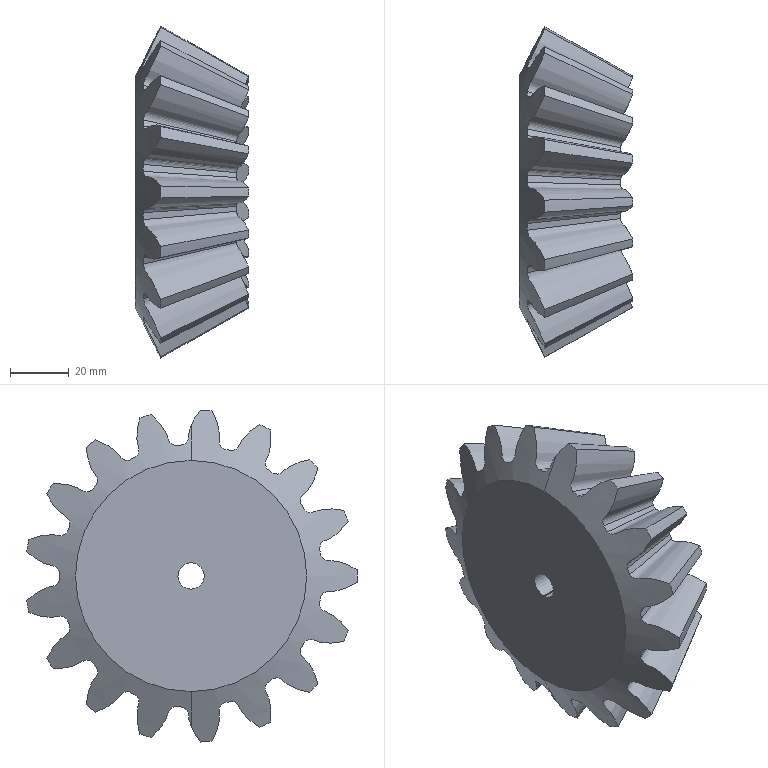Part | STEP file | Bevel gear 17×2 | 1 solid | 94 faces | box 38.391 x 112.113 x 112.556 mm | volume 206962 mm3 | spline 51 | cone 37 | plane 5 | cylinder 1 | commonest cylinder face diameters 8.912 x1